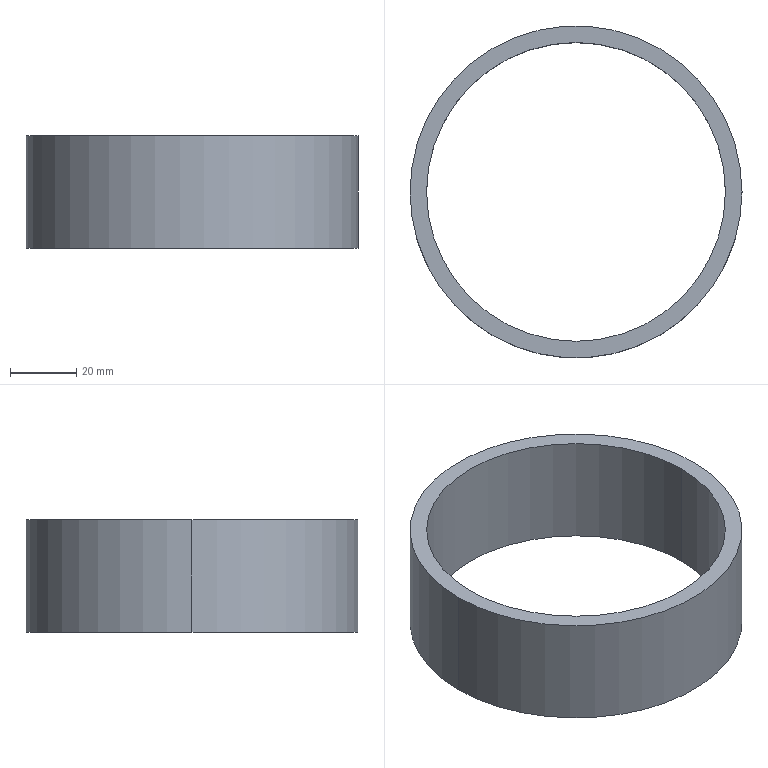Part | SolidWorks | features Extrusion 1 | 1 solid | 6 faces | box 100 x 100 x 34 mm | volume 50737 mm3 | cylinder 4 | plane 2 | commonest cylinder face diameters 90 x2 100 x2
STEP:
#1=CARTESIAN_POINT('',(-45.,0.,34.));
#2=VERTEX_POINT('',#1);
#3=CARTESIAN_POINT('',(45.,0.,34.));
#4=VERTEX_POINT('',#3);
#5=CARTESIAN_POINT('',(0.,0.,34.));
#6=DIRECTION('',(0.,0.,1.));
#7=DIRECTION('',(1.,0.,0.));
#8=AXIS2_PLACEMENT_3D('',#5,#6,#7);
#9=CIRCLE('',#8,45.);
#10=EDGE_CURVE('',#2,#4,#9,.T.);
#11=ORIENTED_EDGE('',*,*,#10,.T.);
#12=CARTESIAN_POINT('',(45.,0.,0.));
#13=VERTEX_POINT('',#12);
#14=CARTESIAN_POINT('',(45.,0.,34.));
#15=DIRECTION('',(0.,0.,-1.));
#16=VECTOR('',#15,1000.);
#17=LINE('',#14,#16);
#18=EDGE_CURVE('',#4,#13,#17,.T.);
#19=ORIENTED_EDGE('',*,*,#18,.T.);
#20=CARTESIAN_POINT('',(-45.,0.,0.));
#21=VERTEX_POINT('',#20);
#22=CARTESIAN_POINT('',(0.,0.,0.));
#23=DIRECTION('',(0.,0.,1.));
#24=DIRECTION('',(1.,0.,0.));
#25=AXIS2_PLACEMENT_3D('',#22,#23,#24);
#26=CIRCLE('',#25,45.);
#27=EDGE_CURVE('',#21,#13,#26,.T.);
#28=ORIENTED_EDGE('',*,*,#27,.F.);
#29=CARTESIAN_POINT('',(-45.,0.,34.));
#30=DIRECTION('',(0.,0.,-1.));
#31=VECTOR('',#30,1000.);
#32=LINE('',#29,#31);
#33=EDGE_CURVE('',#2,#21,#32,.T.);
#34=ORIENTED_EDGE('',*,*,#33,.F.);
#35=EDGE_LOOP('',(#11,#19,#28,#34));
#36=FACE_OUTER_BOUND('',#35,.T.);
#37=CARTESIAN_POINT('',(0.,0.,34.));
#38=DIRECTION('',(0.,0.,-1.));
#39=DIRECTION('',(-1.,0.,0.));
#40=AXIS2_PLACEMENT_3D('',#37,#38,#39);
#41=CYLINDRICAL_SURFACE('',#40,45.);
#42=ADVANCED_FACE('',(#36),#41,.F.);
#43=CARTESIAN_POINT('',(50.,0.,34.));
#44=VERTEX_POINT('',#43);
#45=CARTESIAN_POINT('',(-50.,0.,34.));
#46=VERTEX_POINT('',#45);
#47=CARTESIAN_POINT('',(0.,0.,34.));
#48=DIRECTION('',(0.,0.,1.));
#49=DIRECTION('',(1.,0.,0.));
#50=AXIS2_PLACEMENT_3D('',#47,#48,#49);
#51=CIRCLE('',#50,50.);
#52=EDGE_CURVE('',#44,#46,#51,.T.);
#53=ORIENTED_EDGE('',*,*,#52,.F.);
#54=CARTESIAN_POINT('',(50.,0.,0.));
#55=VERTEX_POINT('',#54);
#56=CARTESIAN_POINT('',(50.,0.,34.));
#57=DIRECTION('',(0.,0.,-1.));
#58=VECTOR('',#57,1000.);
#59=LINE('',#56,#58);
#60=EDGE_CURVE('',#44,#55,#59,.T.);
#61=ORIENTED_EDGE('',*,*,#60,.T.);
#62=CARTESIAN_POINT('',(-50.,0.,0.));
#63=VERTEX_POINT('',#62);
#64=CARTESIAN_POINT('',(0.,0.,0.));
#65=DIRECTION('',(0.,0.,1.));
#66=DIRECTION('',(1.,0.,0.));
#67=AXIS2_PLACEMENT_3D('',#64,#65,#66);
#68=CIRCLE('',#67,50.);
#69=EDGE_CURVE('',#55,#63,#68,.T.);
#70=ORIENTED_EDGE('',*,*,#69,.T.);
#71=CARTESIAN_POINT('',(-50.,0.,34.));
#72=DIRECTION('',(0.,0.,-1.));
#73=VECTOR('',#72,1000.);
#74=LINE('',#71,#73);
#75=EDGE_CURVE('',#46,#63,#74,.T.);
#76=ORIENTED_EDGE('',*,*,#75,.F.);
#77=EDGE_LOOP('',(#53,#61,#70,#76));
#78=FACE_OUTER_BOUND('',#77,.T.);
#79=CARTESIAN_POINT('',(0.,0.,34.));
#80=DIRECTION('',(0.,0.,-1.));
#81=DIRECTION('',(-1.,0.,0.));
#82=AXIS2_PLACEMENT_3D('',#79,#80,#81);
#83=CYLINDRICAL_SURFACE('',#82,50.);
#84=ADVANCED_FACE('',(#78),#83,.T.);
#85=CARTESIAN_POINT('',(0.,0.,34.));
#86=DIRECTION('',(0.,0.,1.));
#87=DIRECTION('',(1.,0.,0.));
#88=AXIS2_PLACEMENT_3D('',#85,#86,#87);
#89=CIRCLE('',#88,50.);
#90=EDGE_CURVE('',#46,#44,#89,.T.);
#91=ORIENTED_EDGE('',*,*,#90,.T.);
#92=ORIENTED_EDGE('',*,*,#52,.T.);
#93=EDGE_LOOP('',(#91,#92));
#94=FACE_OUTER_BOUND('',#93,.T.);
#95=ORIENTED_EDGE('',*,*,#10,.F.);
#96=CARTESIAN_POINT('',(0.,0.,34.));
#97=DIRECTION('',(0.,0.,1.));
#98=DIRECTION('',(1.,0.,0.));
#99=AXIS2_PLACEMENT_3D('',#96,#97,#98);
#100=CIRCLE('',#99,45.);
#101=EDGE_CURVE('',#4,#2,#100,.T.);
#102=ORIENTED_EDGE('',*,*,#101,.F.);
#103=EDGE_LOOP('',(#95,#102));
#104=FACE_BOUND('',#103,.T.);
#105=CARTESIAN_POINT('',(0.,0.,34.));
#106=DIRECTION('',(0.,0.,1.));
#107=DIRECTION('',(1.,0.,0.));
#108=AXIS2_PLACEMENT_3D('',#105,#106,#107);
#109=PLANE('',#108);
#110=ADVANCED_FACE('',(#94,#104),#109,.T.);
#111=CARTESIAN_POINT('',(0.,0.,0.));
#112=DIRECTION('',(0.,0.,1.));
#113=DIRECTION('',(1.,0.,0.));
#114=AXIS2_PLACEMENT_3D('',#111,#112,#113);
#115=CIRCLE('',#114,50.);
#116=EDGE_CURVE('',#63,#55,#115,.T.);
#117=ORIENTED_EDGE('',*,*,#116,.F.);
#118=ORIENTED_EDGE('',*,*,#69,.F.);
#119=EDGE_LOOP('',(#117,#118));
#120=FACE_OUTER_BOUND('',#119,.T.);
#121=ORIENTED_EDGE('',*,*,#27,.T.);
#122=CARTESIAN_POINT('',(0.,0.,0.));
#123=DIRECTION('',(0.,0.,1.));
#124=DIRECTION('',(1.,0.,0.));
#125=AXIS2_PLACEMENT_3D('',#122,#123,#124);
#126=CIRCLE('',#125,45.);
#127=EDGE_CURVE('',#13,#21,#126,.T.);
#128=ORIENTED_EDGE('',*,*,#127,.T.);
#129=EDGE_LOOP('',(#121,#128));
#130=FACE_BOUND('',#129,.T.);
#131=CARTESIAN_POINT('',(0.,0.,0.));
#132=DIRECTION('',(0.,0.,1.));
#133=DIRECTION('',(1.,0.,0.));
#134=AXIS2_PLACEMENT_3D('',#131,#132,#133);
#135=PLANE('',#134);
#136=ADVANCED_FACE('',(#120,#130),#135,.F.);
#137=ORIENTED_EDGE('',*,*,#60,.F.);
#138=ORIENTED_EDGE('',*,*,#90,.F.);
#139=ORIENTED_EDGE('',*,*,#75,.T.);
#140=ORIENTED_EDGE('',*,*,#116,.T.);
#141=EDGE_LOOP('',(#137,#138,#139,#140));
#142=FACE_OUTER_BOUND('',#141,.T.);
#143=CARTESIAN_POINT('',(0.,0.,34.));
#144=DIRECTION('',(0.,0.,-1.));
#145=DIRECTION('',(-1.,0.,0.));
#146=AXIS2_PLACEMENT_3D('',#143,#144,#145);
#147=CYLINDRICAL_SURFACE('',#146,50.);
#148=ADVANCED_FACE('',(#142),#147,.T.);
#149=ORIENTED_EDGE('',*,*,#18,.F.);
#150=ORIENTED_EDGE('',*,*,#101,.T.);
#151=ORIENTED_EDGE('',*,*,#33,.T.);
#152=ORIENTED_EDGE('',*,*,#127,.F.);
#153=EDGE_LOOP('',(#149,#150,#151,#152));
#154=FACE_OUTER_BOUND('',#153,.T.);
#155=CARTESIAN_POINT('',(0.,0.,34.));
#156=DIRECTION('',(0.,0.,-1.));
#157=DIRECTION('',(-1.,0.,0.));
#158=AXIS2_PLACEMENT_3D('',#155,#156,#157);
#159=CYLINDRICAL_SURFACE('',#158,45.);
#160=ADVANCED_FACE('',(#154),#159,.F.);
#161=CLOSED_SHELL('',(#42,#84,#110,#136,#148,#160));
#162=MANIFOLD_SOLID_BREP('',#161);
#163=CARTESIAN_POINT('',(0.,0.,0.));
#164=DIRECTION('',(0.,0.,1.));
#165=DIRECTION('',(1.,0.,0.));
#166=AXIS2_PLACEMENT_3D('',#163,#164,#165);
#167=(LENGTH_UNIT()NAMED_UNIT(*)SI_UNIT(.MILLI.,.METRE.));
#168=UNCERTAINTY_MEASURE_WITH_UNIT(LENGTH_MEASURE(0.00001),#167,'','');
#169=(NAMED_UNIT(*)PLANE_ANGLE_UNIT()SI_UNIT($,.RADIAN.));
#170=(NAMED_UNIT(*)SI_UNIT($,.STERADIAN.)SOLID_ANGLE_UNIT());
#171=(GEOMETRIC_REPRESENTATION_CONTEXT(3)GLOBAL_UNCERTAINTY_ASSIGNED_CONTEXT((#168))GLOBAL_UNIT_ASSIGNED_CONTEXT((#167,#169,#170))REPRESENTATION_CONTEXT('',''));
#172=ADVANCED_BREP_SHAPE_REPRESENTATION('',(#162,#166),#171);